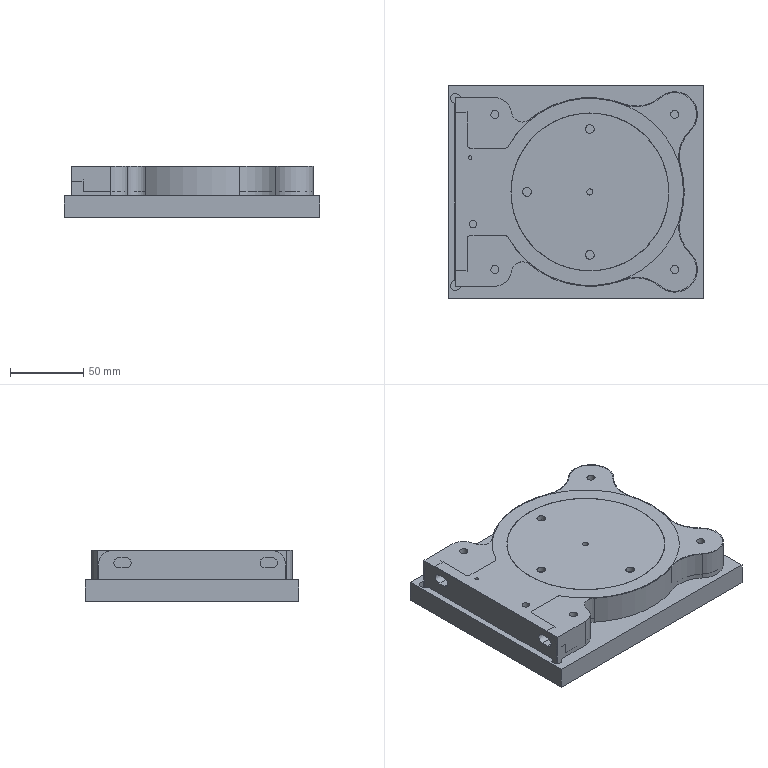NC program | NX | posted with a generic post | part box 175 x 146 x 35 mm
Lines 4709 to 5827 of 35144:
(深度开粗_COPY , TOOL : D6)
N9278 T04 M6
N9280 G54
N9282 G17 G0 G90 X-65.994 Y19.5 S9000 M3
N9284 G43 Z20. H4
N9286 Z0.
N9288 G94 G1 Z-0.5 F2500.
N9290 G3 X-68.994 Y22.5 R3.
N9292 G1 X-71.
N9294 Y20.494
N9296 G3 X-68. Y17.494 R3.
N9298 G1 Z0.
N9300 G0 X-65.994 Y19.5 Z-0.5
N9302 G1 Z-1.
N9304 G3 X-68.994 Y22.5 R3.
N9306 G1 X-71.
N9308 Y20.494
N9310 G3 X-68. Y17.494 R3.
N9312 G1 Z-0.5
N9314 G0 X-65.994 Y19.5 Z-1.
N9316 G1 Z-1.5
N9318 G3 X-68.994 Y22.5 R3.
N9320 G1 X-71.
N9322 Y20.494
N9324 G3 X-68. Y17.494 R3.
N9326 G1 Z-1.
N9328 G0 X-65.994 Y19.5 Z-1.5
N9330 G1 Z-2.
N9332 G3 X-68.994 Y22.5 R3.
N9334 G1 X-71.
N9336 Y20.494
N9338 G3 X-68. Y17.494 R3.
N9340 G1 Z-1.5
N9342 G0 X-65.994 Y19.5 Z-2.
N9344 G1 Z-2.5
N9346 G3 X-68.994 Y22.5 R3.
N9348 G1 X-71.
N9350 Y20.494
N9352 G3 X-68. Y17.494 R3.
N9354 G1 Z-2.
N9356 G0 X-65.994 Y19.5 Z-2.5
N9358 G1 Z-3.
N9360 G3 X-68.994 Y22.5 R3.
N9362 G1 X-71.
N9364 Y20.494
N9366 G3 X-68. Y17.494 R3.
N9368 G1 Z-2.5
N9370 G0 X-65.994 Y19.5 Z-3.
N9372 G1 Z-3.5
N9374 G3 X-68.994 Y22.5 R3.
N9376 G1 X-71.
N9378 Y20.494
N9380 G3 X-68. Y17.494 R3.
N9382 G1 Z-3.
N9384 G0 X-65.994 Y19.5 Z-3.5
N9386 G1 Z-4.
N9388 G3 X-68.994 Y22.5 R3.
N9390 G1 X-71.
N9392 Y20.494
N9394 G3 X-68. Y17.494 R3.
N9396 G1 Z-3.5
N9398 G0 X-65.994 Y19.5 Z-4.
N9400 G1 Z-4.5
N9402 G3 X-68.994 Y22.5 R3.
N9404 G1 X-71.
N9406 Y20.494
N9408 G3 X-68. Y17.494 R3.
N9410 G1 Z-4.
N9412 G0 X-65.994 Y19.5 Z-4.5
N9414 G1 Z-5.
N9416 G3 X-68.994 Y22.5 R3.
N9418 G1 X-71.
N9420 Y20.494
N9422 G3 X-68. Y17.494 R3.
N9424 G1 Z-4.5
N9426 G0 X-65.994 Y19.5 Z-5.
N9428 G1 Z-5.5
N9430 G3 X-68.994 Y22.5 R3.
N9432 G1 X-71.
N9434 Y20.494
N9436 G3 X-68. Y17.494 R3.
N9438 G1 Z-5.
N9440 G0 X-65.994 Y19.5 Z-5.5
N9442 G1 Z-6.
N9444 G3 X-68.994 Y22.5 R3.
N9446 G1 X-71.
N9448 Y20.494
N9450 G3 X-68. Y17.494 R3.
N9452 G1 Z-5.5
N9454 G0 X-65.994 Y19.5 Z-6.
N9456 G1 Z-6.5
N9458 G3 X-68.994 Y22.5 R3.
N9460 G1 X-71.
N9462 Y20.494
N9464 G3 X-68. Y17.494 R3.
N9466 G1 Z-6.
N9468 G0 X-65.994 Y19.5 Z-6.5
N9470 G1 Z-7.
N9472 G3 X-68.994 Y22.5 R3.
N9474 G1 X-71.
N9476 Y20.494
N9478 G3 X-68. Y17.494 R3.
N9480 G1 Z-6.5
N9482 G0 X-65.994 Y19.5 Z-7.
N9484 G1 Z-7.5
N9486 G3 X-68.994 Y22.5 R3.
N9488 G1 X-71.
N9490 Y20.494
N9492 G3 X-68. Y17.494 R3.
N9494 G1 Z-7.
N9496 G0 X-65.994 Y19.5 Z-7.5
N9498 G1 Z-8.
N9500 G3 X-68.994 Y22.5 R3.
N9502 G1 X-71.
N9504 Y20.494
N9506 G3 X-68. Y17.494 R3.
N9508 G1 Z-7.5
N9510 G0 X-65.994 Y19.5 Z-8.
N9512 G1 Z-8.5
N9514 G3 X-68.994 Y22.5 R3.
N9516 G1 X-71.
N9518 Y20.494
N9520 G3 X-68. Y17.494 R3.
N9522 G1 Z-8.
N9524 G0 X-65.994 Y19.5 Z-8.5
N9526 G1 Z-9.
N9528 G3 X-68.994 Y22.5 R3.
N9530 G1 X-71.
N9532 Y20.494
N9534 G3 X-68. Y17.494 R3.
N9536 G1 Z-8.5
N9538 G0 X-65.994 Y19.5 Z-9.
N9540 G1 Z-9.5
N9542 G3 X-68.994 Y22.5 R3.
N9544 G1 X-71.
N9546 Y20.494
N9548 G3 X-68. Y17.494 R3.
N9550 G1 Z-9.
N9552 G0 X-65.994 Y19.5 Z-9.5
N9554 G1 Z-10.
N9556 G3 X-68.994 Y22.5 R3.
N9558 G1 X-71.
N9560 Y20.494
N9562 G3 X-68. Y17.494 R3.
N9564 G1 Z-9.5
N9566 G0 X-65.994 Y19.5 Z-10.
N9568 G1 Z-10.5
N9570 G3 X-68.994 Y22.5 R3.
N9572 G1 X-71.
N9574 Y20.494
N9576 G3 X-68. Y17.494 R3.
N9578 G1 Z-10.
N9580 G0 X-65.994 Y19.5 Z-10.5
N9582 G1 Z-11.
N9584 G3 X-68.994 Y22.5 R3.
N9586 G1 X-71.
N9588 Y20.494
N9590 G3 X-68. Y17.494 R3.
N9592 G1 Z-10.5
N9594 G0 X-65.994 Y19.5 Z-11.
N9596 G1 Z-11.5
N9598 G3 X-68.994 Y22.5 R3.
N9600 G1 X-71.
N9602 Y20.494
N9604 G3 X-68. Y17.494 R3.
N9606 G1 Z-11.
N9608 G0 X-65.994 Y19.5 Z-11.5
N9610 G1 Z-12.
N9612 G3 X-68.994 Y22.5 R3.
N9614 G1 X-71.
N9616 Y20.494
N9618 G3 X-68. Y17.494 R3.
N9620 G1 Z-11.5
N9622 G0 X-65.994 Y19.5 Z-12.
N9624 G1 Z-12.5
N9626 G3 X-68.994 Y22.5 R3.
N9628 G1 X-71.
N9630 Y20.494
N9632 G3 X-68. Y17.494 R3.
N9634 G1 Z-12.
N9636 G0 X-65.994 Y19.5 Z-12.5
N9638 G1 Z-13.
N9640 G3 X-68.994 Y22.5 R3.
N9642 G1 X-71.
N9644 Y20.494
N9646 G3 X-68. Y17.494 R3.
N9648 G1 Z-12.5
N9650 G0 X-65.994 Y19.5 Z-13.
N9652 G1 Z-13.5
N9654 G3 X-68.994 Y22.5 R3.
N9656 G1 X-71.
N9658 Y20.494
N9660 G3 X-68. Y17.494 R3.
N9662 G1 Z-13.
N9664 G0 X-65.994 Y19.5 Z-13.5
N9666 G1 Z-14.
N9668 G3 X-68.994 Y22.5 R3.
N9670 G1 X-71.
N9672 Y20.494
N9674 G3 X-68. Y17.494 R3.
N9676 G1 Z-13.5
N9678 G0 X-65.994 Y19.5 Z-14.
N9680 G1 Z-14.5
N9682 G3 X-68.994 Y22.5 R3.
N9684 G1 X-71.
N9686 Y20.494
N9688 G3 X-68. Y17.494 R3.
N9690 G1 Z-14.
N9692 G0 X-65.994 Y19.5 Z-14.5
N9694 G1 Z-15.
N9696 G3 X-68.994 Y22.5 R3.
N9698 G1 X-71.
N9700 Y20.494
N9702 G3 X-68. Y17.494 R3.
N9704 G1 Z-14.5
N9706 G0 X-65.994 Y19.5 Z-15.
N9708 G1 Z-15.5
N9710 G3 X-68.994 Y22.5 R3.
N9712 G1 X-71.
N9714 Y20.494
N9716 G3 X-68. Y17.494 R3.
N9718 G1 Z-15.
N9720 G0 X-65.994 Y19.5 Z-15.5
N9722 G1 Z-16.
N9724 G3 X-68.994 Y22.5 R3.
N9726 G1 X-71.
N9728 Y20.494
N9730 G3 X-68. Y17.494 R3.
N9732 G1 Z-15.5
N9734 G0 X-65.994 Y19.5 Z-16.
N9736 G1 Z-16.5
N9738 G3 X-68.994 Y22.5 R3.
N9740 G1 X-71.
N9742 Y20.494
N9744 G3 X-68. Y17.494 R3.
N9746 G1 Z-16.
N9748 G0 X-65.994 Y19.5 Z-16.5
N9750 G1 Z-17.
N9752 G3 X-68.994 Y22.5 R3.
N9754 G1 X-71.
N9756 Y20.494
N9758 G3 X-68. Y17.494 R3.
N9760 G1 Z-16.5
N9762 G0 X-65.994 Y19.5 Z-17.
N9764 G1 Z-17.5
N9766 G3 X-68.994 Y22.5 R3.
N9768 G1 X-71.
N9770 Y20.494
N9772 G3 X-68. Y17.494 R3.
N9774 G1 Z-17.
N9776 G0 X-65.994 Y19.5 Z-17.5
N9778 G1 Z-18.
N9780 G3 X-68.994 Y22.5 R3.
N9782 G1 X-71.
N9784 Y20.494
N9786 G3 X-68. Y17.494 R3.
N9788 G1 Z-17.5
N9790 G0 X-65.994 Y19.5 Z-18.
N9792 G1 Z-18.5
N9794 G3 X-68.994 Y22.5 R3.
N9796 G1 X-71.
N9798 Y20.494
N9800 G3 X-68. Y17.494 R3.
N9802 G1 Z-18.
N9804 G0 X-65.994 Y19.5 Z-18.5
N9806 G1 Z-19.
N9808 G3 X-68.994 Y22.5 R3.
N9810 G1 X-71.
N9812 Y20.494
N9814 G3 X-68. Y17.494 R3.
N9816 G1 Z-18.5
N9818 G0 X-65.994 Y19.5 Z-18.8
N9820 G1 Z-19.3
N9822 G3 X-68.994 Y22.5 R3.
N9824 G1 X-71.
N9826 Y20.494
N9828 G3 X-68. Y17.494 R3.
N9830 G1 Z-18.8
N9832 G0 X-65.994 Y11.523 Z-19.15
N9834 G1 Z-19.65
N9836 G3 X-68.994 Y14.523 R3.
N9838 G1 X-71.
N9840 Y12.517
N9842 G3 X-68. Y9.517 R3.
N9844 G1 Z-19.15
N9846 G0 X-65.994 Y11.5 Z-19.5
N9848 G1 Z-20.
N9850 G3 X-68.994 Y14.5 R3.
N9852 G1 X-71.
N9854 Y12.494
N9856 G3 X-68. Y9.494 R3.
N9858 G1 Z-19.5
N9860 G0 Z20.
N9862 X-62. Y17.494
N9864 Z-1.
N9866 G1 Z-1.5
N9868 G3 X-59. Y20.494 R3.
N9870 G1 Y22.5
N9872 X-61.006
N9874 G3 X-64.006 Y19.5 R3.
N9876 G1 Z-1.
N9878 G0 X-62. Y17.494 Z-1.5
N9880 G1 Z-2.
N9882 G3 X-59. Y20.494 R3.
N9884 G1 Y22.5
N9886 X-61.006
N9888 G3 X-64.006 Y19.5 R3.
N9890 G1 Z-1.5
N9892 G0 X-62. Y17.494 Z-2.
N9894 G1 Z-2.5
N9896 G3 X-59. Y20.494 R3.
N9898 G1 Y22.5
N9900 X-61.006
N9902 G3 X-64.006 Y19.5 R3.
N9904 G1 Z-2.
N9906 G0 X-62. Y17.494 Z-2.5
N9908 G1 Z-3.
N9910 G3 X-59. Y20.494 R3.
N9912 G1 Y22.5
N9914 X-61.006
N9916 G3 X-64.006 Y19.5 R3.
N9918 G1 Z-2.5
N9920 G0 X-62. Y17.494 Z-3.
N9922 G1 Z-3.5
N9924 G3 X-59. Y20.494 R3.
N9926 G1 Y22.5
N9928 X-61.006
N9930 G3 X-64.006 Y19.5 R3.
N9932 G1 Z-3.
N9934 G0 X-62. Y17.494 Z-3.5
N9936 G1 Z-4.
N9938 G3 X-59. Y20.494 R3.
N9940 G1 Y22.5
N9942 X-61.006
N9944 G3 X-64.006 Y19.5 R3.
N9946 G1 Z-3.5
N9948 G0 X-62. Y17.494 Z-4.
N9950 G1 Z-4.5
N9952 G3 X-59. Y20.494 R3.
N9954 G1 Y22.5
N9956 X-61.006
N9958 G3 X-64.006 Y19.5 R3.
N9960 G1 Z-4.
N9962 G0 X-62. Y17.494 Z-4.5
N9964 G1 Z-5.
N9966 G3 X-59. Y20.494 R3.
N9968 G1 Y22.5
N9970 X-61.006
N9972 G3 X-64.006 Y19.5 R3.
N9974 G1 Z-4.5
N9976 G0 X-62. Y17.494 Z-5.
N9978 G1 Z-5.5
N9980 G3 X-59. Y20.494 R3.
N9982 G1 Y22.5
N9984 X-61.006
N9986 G3 X-64.006 Y19.5 R3.
N9988 G1 Z-5.
N9990 G0 X-62. Y17.494 Z-5.5
N9992 G1 Z-6.
N9994 G3 X-59. Y20.494 R3.
N9996 G1 Y22.5
N9998 X-61.006
N10000 G3 X-64.006 Y19.5 R3.
N10002 G1 Z-5.5
N10004 G0 X-62. Y17.494 Z-6.
N10006 G1 Z-6.5
N10008 G3 X-59. Y20.494 R3.
N10010 G1 Y22.5
N10012 X-61.006
N10014 G3 X-64.006 Y19.5 R3.
N10016 G1 Z-6.
N10018 G0 X-62. Y17.494 Z-6.5
N10020 G1 Z-7.
N10022 G3 X-59. Y20.494 R3.
N10024 G1 Y22.5
N10026 X-61.006
N10028 G3 X-64.006 Y19.5 R3.
N10030 G1 Z-6.5
N10032 G0 X-62. Y17.494 Z-7.
N10034 G1 Z-7.5
N10036 G3 X-59. Y20.494 R3.
N10038 G1 Y22.5
N10040 X-61.006
N10042 G3 X-64.006 Y19.5 R3.
N10044 G1 Z-7.
N10046 G0 X-62. Y17.494 Z-7.5
N10048 G1 Z-8.
N10050 G3 X-59. Y20.494 R3.
N10052 G1 Y22.5
N10054 X-61.006
N10056 G3 X-64.006 Y19.5 R3.
N10058 G1 Z-7.5
N10060 G0 X-62. Y17.494 Z-8.
N10062 G1 Z-8.5
N10064 G3 X-59. Y20.494 R3.
N10066 G1 Y22.5
N10068 X-61.006
N10070 G3 X-64.006 Y19.5 R3.
N10072 G1 Z-8.
N10074 G0 X-62. Y17.494 Z-8.5
N10076 G1 Z-9.
N10078 G3 X-59. Y20.494 R3.
N10080 G1 Y22.5
N10082 X-61.006
N10084 G3 X-64.006 Y19.5 R3.
N10086 G1 Z-8.5
N10088 G0 X-62. Y17.494 Z-9.
N10090 G1 Z-9.5
N10092 G3 X-59. Y20.494 R3.
N10094 G1 Y22.5
N10096 X-61.006
N10098 G3 X-64.006 Y19.5 R3.
N10100 G1 Z-9.
N10102 G0 X-62. Y17.494 Z-9.5
N10104 G1 Z-10.
N10106 G3 X-59. Y20.494 R3.
N10108 G1 Y22.5
N10110 X-61.006
N10112 G3 X-64.006 Y19.5 R3.
N10114 G1 Z-9.5
N10116 G0 X-62. Y17.494 Z-10.
N10118 G1 Z-10.5
N10120 G3 X-59. Y20.494 R3.
N10122 G1 Y22.5
N10124 X-61.006
N10126 G3 X-64.006 Y19.5 R3.
N10128 G1 Z-10.
N10130 G0 X-62. Y17.494 Z-10.5
N10132 G1 Z-11.
N10134 G3 X-59. Y20.494 R3.
N10136 G1 Y22.5
N10138 X-61.006
N10140 G3 X-64.006 Y19.5 R3.
N10142 G1 Z-10.5
N10144 G0 X-62. Y17.494 Z-11.
N10146 G1 Z-11.5
N10148 G3 X-59. Y20.494 R3.
N10150 G1 Y22.5
N10152 X-61.006
N10154 G3 X-64.006 Y19.5 R3.
N10156 G1 Z-11.
N10158 G0 X-62. Y17.494 Z-11.5
N10160 G1 Z-12.
N10162 G3 X-59. Y20.494 R3.
N10164 G1 Y22.5
N10166 X-61.006
N10168 G3 X-64.006 Y19.5 R3.
N10170 G1 Z-11.5
N10172 G0 X-62. Y17.494 Z-12.
N10174 G1 Z-12.5
N10176 G3 X-59. Y20.494 R3.
N10178 G1 Y22.5
N10180 X-61.006
N10182 G3 X-64.006 Y19.5 R3.
N10184 G1 Z-12.
N10186 G0 X-62. Y17.494 Z-12.5
N10188 G1 Z-13.
N10190 G3 X-59. Y20.494 R3.
N10192 G1 Y22.5
N10194 X-61.006
N10196 G3 X-64.006 Y19.5 R3.
N10198 G1 Z-12.5
N10200 G0 X-62. Y17.494 Z-13.
N10202 G1 Z-13.5
N10204 G3 X-59. Y20.494 R3.
N10206 G1 Y22.5
N10208 X-61.006
N10210 G3 X-64.006 Y19.5 R3.
N10212 G1 Z-13.
N10214 G0 X-62. Y17.494 Z-13.5
N10216 G1 Z-14.
N10218 G3 X-59. Y20.494 R3.
N10220 G1 Y22.5
N10222 X-61.006
N10224 G3 X-64.006 Y19.5 R3.
N10226 G1 Z-13.5
N10228 G0 X-62. Y17.494 Z-14.
N10230 G1 Z-14.5
N10232 G3 X-59. Y20.494 R3.
N10234 G1 Y22.5
N10236 X-61.006
N10238 G3 X-64.006 Y19.5 R3.
N10240 G1 Z-14.
N10242 G0 X-62. Y17.494 Z-14.5
N10244 G1 Z-15.
N10246 G3 X-59. Y20.494 R3.
N10248 G1 Y22.5
N10250 X-61.006
N10252 G3 X-64.006 Y19.5 R3.
N10254 G1 Z-14.5
N10256 G0 X-62. Y17.494 Z-15.
N10258 G1 Z-15.5
N10260 G3 X-59. Y20.494 R3.
N10262 G1 Y22.5
N10264 X-61.006
N10266 G3 X-64.006 Y19.5 R3.
N10268 G1 Z-15.
N10270 G0 X-62. Y17.494 Z-15.5
N10272 G1 Z-16.
N10274 G3 X-59. Y20.494 R3.
N10276 G1 Y22.5
N10278 X-61.006
N10280 G3 X-64.006 Y19.5 R3.
N10282 G1 Z-15.5
N10284 G0 X-62. Y17.494 Z-16.
N10286 G1 Z-16.5
N10288 G3 X-59. Y20.494 R3.
N10290 G1 Y22.5
N10292 X-61.006
N10294 G3 X-64.006 Y19.5 R3.
N10296 G1 Z-16.
N10298 G0 X-62. Y17.494 Z-16.5
N10300 G1 Z-17.
N10302 G3 X-59. Y20.494 R3.
N10304 G1 Y22.5
N10306 X-61.006
N10308 G3 X-64.006 Y19.5 R3.
N10310 G1 Z-16.5
N10312 G0 X-62. Y17.494 Z-17.
N10314 G1 Z-17.5
N10316 G3 X-59. Y20.494 R3.
N10318 G1 Y22.5
N10320 X-61.006
N10322 G3 X-64.006 Y19.5 R3.
N10324 G1 Z-17.
N10326 G0 X-62. Y17.494 Z-17.5
N10328 G1 Z-18.
N10330 G3 X-59. Y20.494 R3.
N10332 G1 Y22.5
N10334 X-61.006
N10336 G3 X-64.006 Y19.5 R3.
N10338 G1 Z-17.5
N10340 G0 X-62. Y17.494 Z-18.
N10342 G1 Z-18.5
N10344 G3 X-59. Y20.494 R3.
N10346 G1 Y22.5
N10348 X-61.006
N10350 G3 X-64.006 Y19.5 R3.
N10352 G1 Z-18.
N10354 G0 X-62. Y17.494 Z-18.5
N10356 G1 Z-19.
N10358 G3 X-59. Y20.494 R3.
N10360 G1 Y22.5
N10362 X-61.006
N10364 G3 X-64.006 Y19.5 R3.
N10366 G1 Z-18.5
N10368 G0 X-62. Y17.494 Z-18.8
N10370 G1 Z-19.3
N10372 G3 X-59. Y20.494 R3.
N10374 G1 Y22.5
N10376 X-61.006
N10378 G3 X-64.006 Y19.5 R3.
N10380 G1 Z-18.8
N10382 G0 X-62. Y17.141 Z-19.15
N10384 G1 Z-19.65
N10386 G3 X-59. Y20.141 R3.
N10388 G1 Y22.5
N10390 X-63.023
N10392 Y20.141
N10394 G3 X-60.023 Y17.141 R3.
N10396 G1 Z-19.15
N10398 G0 X-62. Y14.906 Z-19.5
N10400 G1 Z-20.
N10402 G3 X-59. Y17.906 R3.
N10404 G1 Y22.5
N10406 X-63.
N10408 Y18.335
N10410 G3 X-60. Y15.335 R3.
N10412 G1 Z-19.5
N10414 G0 Z20.
N10416 X-68. Y-17.494
N10418 Z0.
N10420 G1 Z-0.5
N10422 G3 X-71. Y-20.494 R3.
N10424 G1 Y-22.5
N10426 X-68.994
N10428 G3 X-65.994 Y-19.5 R3.
N10430 G1 Z0.
N10432 G0 X-68. Y-17.494 Z-0.5
N10434 G1 Z-1.
N10436 G3 X-71. Y-20.494 R3.
N10438 G1 Y-22.5
N10440 X-68.994
N10442 G3 X-65.994 Y-19.5 R3.
N10444 G1 Z-0.5
N10446 G0 X-68. Y-17.494 Z-1.
N10448 G1 Z-1.5
N10450 G3 X-71. Y-20.494 R3.
N10452 G1 Y-22.5
N10454 X-68.994
N10456 G3 X-65.994 Y-19.5 R3.
N10458 G1 Z-1.
N10460 G0 X-68. Y-17.494 Z-1.5
N10462 G1 Z-2.
N10464 G3 X-71. Y-20.494 R3.
N10466 G1 Y-22.5
N10468 X-68.994
N10470 G3 X-65.994 Y-19.5 R3.
N10472 G1 Z-1.5
N10474 G0 X-68. Y-17.494 Z-2.
N10476 G1 Z-2.5
N10478 G3 X-71. Y-20.494 R3.
N10480 G1 Y-22.5
N10482 X-68.994
N10484 G3 X-65.994 Y-19.5 R3.
N10486 G1 Z-2.
N10488 G0 X-68. Y-17.494 Z-2.5
N10490 G1 Z-3.
N10492 G3 X-71. Y-20.494 R3.
N10494 G1 Y-22.5
N10496 X-68.994
N10498 G3 X-65.994 Y-19.5 R3.
N10500 G1 Z-2.5
N10502 G0 X-68. Y-17.494 Z-3.
N10504 G1 Z-3.5
N10506 G3 X-71. Y-20.494 R3.
N10508 G1 Y-22.5
N10510 X-68.994
N10512 G3 X-65.994 Y-19.5 R3.
N10514 G1 Z-3.
N10516 G0 X-68. Y-17.494 Z-3.5
N10518 G1 Z-4.
N10520 G3 X-71. Y-20.494 R3.
N10522 G1 Y-22.5
N10524 X-68.994
N10526 G3 X-65.994 Y-19.5 R3.
N10528 G1 Z-3.5
N10530 G0 X-68. Y-17.494 Z-4.
N10532 G1 Z-4.5
N10534 G3 X-71. Y-20.494 R3.
N10536 G1 Y-22.5
N10538 X-68.994
N10540 G3 X-65.994 Y-19.5 R3.
N10542 G1 Z-4.
N10544 G0 X-68. Y-17.494 Z-4.5
N10546 G1 Z-5.
N10548 G3 X-71. Y-20.494 R3.
N10550 G1 Y-22.5
N10552 X-68.994
N10554 G3 X-65.994 Y-19.5 R3.
N10556 G1 Z-4.5
N10558 G0 X-68. Y-17.494 Z-5.
N10560 G1 Z-5.5
N10562 G3 X-71. Y-20.494 R3.
N10564 G1 Y-22.5
N10566 X-68.994
N10568 G3 X-65.994 Y-19.5 R3.
N10570 G1 Z-5.
N10572 G0 X-68. Y-17.494 Z-5.5
N10574 G1 Z-6.
N10576 G3 X-71. Y-20.494 R3.
N10578 G1 Y-22.5
N10580 X-68.994
N10582 G3 X-65.994 Y-19.5 R3.
N10584 G1 Z-5.5
N10586 G0 X-68. Y-17.494 Z-6.
N10588 G1 Z-6.5
N10590 G3 X-71. Y-20.494 R3.
N10592 G1 Y-22.5
N10594 X-68.994
N10596 G3 X-65.994 Y-19.5 R3.
N10598 G1 Z-6.
N10600 G0 X-68. Y-17.494 Z-6.5
N10602 G1 Z-7.
N10604 G3 X-71. Y-20.494 R3.
N10606 G1 Y-22.5
N10608 X-68.994
N10610 G3 X-65.994 Y-19.5 R3.
N10612 G1 Z-6.5
N10614 G0 X-68. Y-17.494 Z-7.
N10616 G1 Z-7.5
N10618 G3 X-71. Y-20.494 R3.
N10620 G1 Y-22.5
N10622 X-68.994
N10624 G3 X-65.994 Y-19.5 R3.
N10626 G1 Z-7.
N10628 G0 X-68. Y-17.494 Z-7.5
N10630 G1 Z-8.
N10632 G3 X-71. Y-20.494 R3.
N10634 G1 Y-22.5
N10636 X-68.994
N10638 G3 X-65.994 Y-19.5 R3.
N10640 G1 Z-7.5
N10642 G0 X-68. Y-17.494 Z-8.
N10644 G1 Z-8.5
N10646 G3 X-71. Y-20.494 R3.
N10648 G1 Y-22.5
N10650 X-68.994
N10652 G3 X-65.994 Y-19.5 R3.
N10654 G1 Z-8.
N10656 G0 X-68. Y-17.494 Z-8.5
N10658 G1 Z-9.
N10660 G3 X-71. Y-20.494 R3.
N10662 G1 Y-22.5
N10664 X-68.994
N10666 G3 X-65.994 Y-19.5 R3.
N10668 G1 Z-8.5
N10670 G0 X-68. Y-17.494 Z-9.
N10672 G1 Z-9.5
N10674 G3 X-71. Y-20.494 R3.
N10676 G1 Y-22.5
N10678 X-68.994
N10680 G3 X-65.994 Y-19.5 R3.
N10682 G1 Z-9.
N10684 G0 X-68. Y-17.494 Z-9.5
N10686 G1 Z-10.
N10688 G3 X-71. Y-20.494 R3.
N10690 G1 Y-22.5
N10692 X-68.994
N10694 G3 X-65.994 Y-19.5 R3.
N10696 G1 Z-9.5
N10698 G0 X-68. Y-17.494 Z-10.
N10700 G1 Z-10.5
N10702 G3 X-71. Y-20.494 R3.
N10704 G1 Y-22.5
N10706 X-68.994
N10708 G3 X-65.994 Y-19.5 R3.
N10710 G1 Z-10.
N10712 G0 X-68. Y-17.494 Z-10.5
N10714 G1 Z-11.
N10716 G3 X-71. Y-20.494 R3.
N10718 G1 Y-22.5
N10720 X-68.994
N10722 G3 X-65.994 Y-19.5 R3.
N10724 G1 Z-10.5
N10726 G0 X-68. Y-17.494 Z-11.
N10728 G1 Z-11.5
N10730 G3 X-71. Y-20.494 R3.
N10732 G1 Y-22.5
N10734 X-68.994
N10736 G3 X-65.994 Y-19.5 R3.
N10738 G1 Z-11.
N10740 G0 X-68. Y-17.494 Z-11.5
N10742 G1 Z-12.
N10744 G3 X-71. Y-20.494 R3.
N10746 G1 Y-22.5
N10748 X-68.994
N10750 G3 X-65.994 Y-19.5 R3.
N10752 G1 Z-11.5
N10754 G0 X-68. Y-17.494 Z-12.
N10756 G1 Z-12.5
N10758 G3 X-71. Y-20.494 R3.
N10760 G1 Y-22.5
N10762 X-68.994
N10764 G3 X-65.994 Y-19.5 R3.
N10766 G1 Z-12.
N10768 G0 X-68. Y-17.494 Z-12.5
N10770 G1 Z-13.
N10772 G3 X-71. Y-20.494 R3.
N10774 G1 Y-22.5
N10776 X-68.994
N10778 G3 X-65.994 Y-19.5 R3.
N10780 G1 Z-12.5
N10782 G0 X-68. Y-17.494 Z-13.
N10784 G1 Z-13.5
N10786 G3 X-71. Y-20.494 R3.
N10788 G1 Y-22.5
N10790 X-68.994
N10792 G3 X-65.994 Y-19.5 R3.
N10794 G1 Z-13.
N10796 G0 X-68. Y-17.494 Z-13.5
N10798 G1 Z-14.
N10800 G3 X-71. Y-20.494 R3.
N10802 G1 Y-22.5
N10804 X-68.994
N10806 G3 X-65.994 Y-19.5 R3.
N10808 G1 Z-13.5
N10810 G0 X-68. Y-17.494 Z-14.
N10812 G1 Z-14.5
N10814 G3 X-71. Y-20.494 R3.
N10816 G1 Y-22.5
N10818 X-68.994
N10820 G3 X-65.994 Y-19.5 R3.
N10822 G1 Z-14.
N10824 G0 X-68. Y-17.494 Z-14.5
N10826 G1 Z-15.
N10828 G3 X-71. Y-20.494 R3.
N10830 G1 Y-22.5
N10832 X-68.994
N10834 G3 X-65.994 Y-19.5 R3.
N10836 G1 Z-14.5
N10838 G0 X-68. Y-17.494 Z-15.
N10840 G1 Z-15.5
N10842 G3 X-71. Y-20.494 R3.
N10844 G1 Y-22.5
N10846 X-68.994
N10848 G3 X-65.994 Y-19.5 R3.
N10850 G1 Z-15.
N10852 G0 X-68. Y-17.494 Z-15.5
N10854 G1 Z-16.
N10856 G3 X-71. Y-20.494 R3.
N10858 G1 Y-22.5
N10860 X-68.994
N10862 G3 X-65.994 Y-19.5 R3.
N10864 G1 Z-15.5
N10866 G0 X-68. Y-17.494 Z-16.
N10868 G1 Z-16.5
N10870 G3 X-71. Y-20.494 R3.
N10872 G1 Y-22.5
N10874 X-68.994
N10876 G3 X-65.994 Y-19.5 R3.
N10878 G1 Z-16.
N10880 G0 X-68. Y-17.494 Z-16.5
N10882 G1 Z-17.
N10884 G3 X-71. Y-20.494 R3.
N10886 G1 Y-22.5
N10888 X-68.994
N10890 G3 X-65.994 Y-19.5 R3.
N10892 G1 Z-16.5
N10894 G0 X-68. Y-17.494 Z-17.
N10896 G1 Z-17.5
N10898 G3 X-71. Y-20.494 R3.
N10900 G1 Y-22.5
N10902 X-68.994
N10904 G3 X-65.994 Y-19.5 R3.
N10906 G1 Z-17.
N10908 G0 X-68. Y-17.494 Z-17.5
N10910 G1 Z-18.
N10912 G3 X-71. Y-20.494 R3.
N10914 G1 Y-22.5
N10916 X-68.994
N10918 G3 X-65.994 Y-19.5 R3.
N10920 G1 Z-17.5
N10922 G0 X-68. Y-17.494 Z-18.
N10924 G1 Z-18.5
N10926 G3 X-71. Y-20.494 R3.
N10928 G1 Y-22.5
N10930 X-68.994
N10932 G3 X-65.994 Y-19.5 R3.
N10934 G1 Z-18.
N10936 G0 X-68. Y-17.494 Z-18.5
N10938 G1 Z-19.
N10940 G3 X-71. Y-20.494 R3.
N10942 G1 Y-22.5
N10944 X-68.994
N10946 G3 X-65.994 Y-19.5 R3.
N10948 G1 Z-18.5
N10950 G0 X-68. Y-17.494 Z-18.8
N10952 G1 Z-19.3
N10954 G3 X-71. Y-20.494 R3.
N10956 G1 Y-22.5
N10958 X-68.994
N10960 G3 X-65.994 Y-19.5 R3.
N10962 G1 Z-18.8
N10964 G0 X-68. Y-17.494 Z-19.15
N10966 G1 Z-19.65
N10968 G3 X-71. Y-20.494 R3.
N10970 G1 Y-22.5
N10972 X-68.994
N10974 G3 X-65.994 Y-19.5 R3.
N10976 G1 Z-19.15
N10978 G0 X-68. Y-17.494 Z-19.5
N10980 G1 Z-20.
N10982 G3 X-71. Y-20.494 R3.
N10984 G1 Y-22.5
N10986 X-68.994
N10988 G3 X-65.994 Y-19.5 R3.
N10990 G1 Z-19.5
N10992 G0 Z20.
N10994 X-64.006
N10996 Z-1.
N10998 G1 Z-1.5
N11000 G3 X-61.006 Y-22.5 R3.
N11002 G1 X-59.
N11004 Y-20.494
N11006 G3 X-62. Y-17.494 R3.
N11008 G1 Z-1.
N11010 G0 X-64.006 Y-19.5 Z-1.5
N11012 G1 Z-2.
N11014 G3 X-61.006 Y-22.5 R3.
N11016 G1 X-59.
N11018 Y-20.494
N11020 G3 X-62. Y-17.494 R3.
N11022 G1 Z-1.5
N11024 G0 X-64.006 Y-19.5 Z-2.
N11026 G1 Z-2.5
N11028 G3 X-61.006 Y-22.5 R3.
N11030 G1 X-59.
N11032 Y-20.494
N11034 G3 X-62. Y-17.494 R3.
N11036 G1 Z-2.
N11038 G0 X-64.006 Y-19.5 Z-2.5
N11040 G1 Z-3.
N11042 G3 X-61.006 Y-22.5 R3.
N11044 G1 X-59.
N11046 Y-20.494
N11048 G3 X-62. Y-17.494 R3.
N11050 G1 Z-2.5
N11052 G0 X-64.006 Y-19.5 Z-3.
N11054 G1 Z-3.5
N11056 G3 X-61.006 Y-22.5 R3.
N11058 G1 X-59.
N11060 Y-20.494
N11062 G3 X-62. Y-17.494 R3.
N11064 G1 Z-3.
N11066 G0 X-64.006 Y-19.5 Z-3.5
N11068 G1 Z-4.
N11070 G3 X-61.006 Y-22.5 R3.
N11072 G1 X-59.
N11074 Y-20.494
N11076 G3 X-62. Y-17.494 R3.
N11078 G1 Z-3.5
N11080 G0 X-64.006 Y-19.5 Z-4.
N11082 G1 Z-4.5
N11084 G3 X-61.006 Y-22.5 R3.
N11086 G1 X-59.
N11088 Y-20.494
N11090 G3 X-62. Y-17.494 R3.
N11092 G1 Z-4.
N11094 G0 X-64.006 Y-19.5 Z-4.5
N11096 G1 Z-5.
N11098 G3 X-61.006 Y-22.5 R3.
N11100 G1 X-59.
N11102 Y-20.494
N11104 G3 X-62. Y-17.494 R3.
N11106 G1 Z-4.5
N11108 G0 X-64.006 Y-19.5 Z-5.
N11110 G1 Z-5.5
N11112 G3 X-61.006 Y-22.5 R3.
N11114 G1 X-59.
N11116 Y-20.494
N11118 G3 X-62. Y-17.494 R3.
N11120 G1 Z-5.
N11122 G0 X-64.006 Y-19.5 Z-5.5
N11124 G1 Z-6.
N11126 G3 X-61.006 Y-22.5 R3.
N11128 G1 X-59.
N11130 Y-20.494
N11132 G3 X-62. Y-17.494 R3.
N11134 G1 Z-5.5
N11136 G0 X-64.006 Y-19.5 Z-6.
N11138 G1 Z-6.5
N11140 G3 X-61.006 Y-22.5 R3.
N11142 G1 X-59.
N11144 Y-20.494
N11146 G3 X-62. Y-17.494 R3.
N11148 G1 Z-6.
N11150 G0 X-64.006 Y-19.5 Z-6.5
N11152 G1 Z-7.
N11154 G3 X-61.006 Y-22.5 R3.
N11156 G1 X-59.
N11158 Y-20.494
N11160 G3 X-62. Y-17.494 R3.
N11162 G1 Z-6.5
N11164 G0 X-64.006 Y-19.5 Z-7.
N11166 G1 Z-7.5
N11168 G3 X-61.006 Y-22.5 R3.
N11170 G1 X-59.
N11172 Y-20.494
N11174 G3 X-62. Y-17.494 R3.
N11176 G1 Z-7.
N11178 G0 X-64.006 Y-19.5 Z-7.5
N11180 G1 Z-8.
N11182 G3 X-61.006 Y-22.5 R3.
N11184 G1 X-59.
N11186 Y-20.494
N11188 G3 X-62. Y-17.494 R3.
N11190 G1 Z-7.5
N11192 G0 X-64.006 Y-19.5 Z-8.
N11194 G1 Z-8.5
N11196 G3 X-61.006 Y-22.5 R3.
N11198 G1 X-59.
N11200 Y-20.494
N11202 G3 X-62. Y-17.494 R3.
N11204 G1 Z-8.
N11206 G0 X-64.006 Y-19.5 Z-8.5
N11208 G1 Z-9.
N11210 G3 X-61.006 Y-22.5 R3.
N11212 G1 X-59.
N11214 Y-20.494
N11216 G3 X-62. Y-17.494 R3.
N11218 G1 Z-8.5
N11220 G0 X-64.006 Y-19.5 Z-9.
N11222 G1 Z-9.5
N11224 G3 X-61.006 Y-22.5 R3.
N11226 G1 X-59.
N11228 Y-20.494
N11230 G3 X-62. Y-17.494 R3.
N11232 G1 Z-9.
N11234 G0 X-64.006 Y-19.5 Z-9.5
N11236 G1 Z-10.
N11238 G3 X-61.006 Y-22.5 R3.
N11240 G1 X-59.
N11242 Y-20.494
N11244 G3 X-62. Y-17.494 R3.
N11246 G1 Z-9.5
N11248 G0 X-64.006 Y-19.5 Z-10.
N11250 G1 Z-10.5
N11252 G3 X-61.006 Y-22.5 R3.
N11254 G1 X-59.
N11256 Y-20.494
N11258 G3 X-62. Y-17.494 R3.
N11260 G1 Z-10.
N11262 G0 X-64.006 Y-19.5 Z-10.5
N11264 G1 Z-11.
N11266 G3 X-61.006 Y-22.5 R3.
N11268 G1 X-59.
N11270 Y-20.494
N11272 G3 X-62. Y-17.494 R3.
N11274 G1 Z-10.5
N11276 G0 X-64.006 Y-19.5 Z-11.
N11278 G1 Z-11.5
N11280 G3 X-61.006 Y-22.5 R3.
N11282 G1 X-59.
N11284 Y-20.494
N11286 G3 X-62. Y-17.494 R3.
N11288 G1 Z-11.
N11290 G0 X-64.006 Y-19.5 Z-11.5
N11292 G1 Z-12.
N11294 G3 X-61.006 Y-22.5 R3.
N11296 G1 X-59.
N11298 Y-20.494
N11300 G3 X-62. Y-17.494 R3.
N11302 G1 Z-11.5
N11304 G0 X-64.006 Y-19.5 Z-12.
N11306 G1 Z-12.5
N11308 G3 X-61.006 Y-22.5 R3.
N11310 G1 X-59.
N11312 Y-20.494
N11314 G3 X-62. Y-17.494 R3.
N11316 G1 Z-12.
N11318 G0 X-64.006 Y-19.5 Z-12.5
N11320 G1 Z-13.
N11322 G3 X-61.006 Y-22.5 R3.
N11324 G1 X-59.
N11326 Y-20.494
N11328 G3 X-62. Y-17.494 R3.
N11330 G1 Z-12.5
N11332 G0 X-64.006 Y-19.5 Z-13.
N11334 G1 Z-13.5
N11336 G3 X-61.006 Y-22.5 R3.
N11338 G1 X-59.
N11340 Y-20.494
N11342 G3 X-62. Y-17.494 R3.
N11344 G1 Z-13.
N11346 G0 X-64.006 Y-19.5 Z-13.5
N11348 G1 Z-14.
N11350 G3 X-61.006 Y-22.5 R3.
N11352 G1 X-59.
N11354 Y-20.494
N11356 G3 X-62. Y-17.494 R3.
N11358 G1 Z-13.5
N11360 G0 X-64.006 Y-19.5 Z-14.
N11362 G1 Z-14.5
N11364 G3 X-61.006 Y-22.5 R3.
N11366 G1 X-59.
N11368 Y-20.494
N11370 G3 X-62. Y-17.494 R3.
N11372 G1 Z-14.
N11374 G0 X-64.006 Y-19.5 Z-14.5
N11376 G1 Z-15.
N11378 G3 X-61.006 Y-22.5 R3.
N11380 G1 X-59.
N11382 Y-20.494
N11384 G3 X-62. Y-17.494 R3.
N11386 G1 Z-14.5
N11388 G0 X-64.006 Y-19.5 Z-15.
N11390 G1 Z-15.5
N11392 G3 X-61.006 Y-22.5 R3.
N11394 G1 X-59.
N11396 Y-20.494
N11398 G3 X-62. Y-17.494 R3.
N11400 G1 Z-15.
N11402 G0 X-64.006 Y-19.5 Z-15.5
N11404 G1 Z-16.
N11406 G3 X-61.006 Y-22.5 R3.
N11408 G1 X-59.
N11410 Y-20.494
N11412 G3 X-62. Y-17.494 R3.
N11414 G1 Z-15.5
N11416 G0 X-64.006 Y-19.5 Z-16.
N11418 G1 Z-16.5
N11420 G3 X-61.006 Y-22.5 R3.
N11422 G1 X-59.
N11424 Y-20.494
N11426 G3 X-62. Y-17.494 R3.
N11428 G1 Z-16.
N11430 G0 X-64.006 Y-19.5 Z-16.5
N11432 G1 Z-17.
N11434 G3 X-61.006 Y-22.5 R3.
N11436 G1 X-59.
N11438 Y-20.494
N11440 G3 X-62. Y-17.494 R3.
N11442 G1 Z-16.5
N11444 G0 X-64.006 Y-19.5 Z-17.
N11446 G1 Z-17.5
N11448 G3 X-61.006 Y-22.5 R3.
N11450 G1 X-59.
N11452 Y-20.494
N11454 G3 X-62. Y-17.494 R3.
N11456 G1 Z-17.
N11458 G0 X-64.006 Y-19.5 Z-17.5
N11460 G1 Z-18.
N11462 G3 X-61.006 Y-22.5 R3.
N11464 G1 X-59.
N11466 Y-20.494
N11468 G3 X-62. Y-17.494 R3.
N11470 G1 Z-17.5
N11472 G0 X-64.006 Y-19.5 Z-18.
N11474 G1 Z-18.5
N11476 G3 X-61.006 Y-22.5 R3.
N11478 G1 X-59.
N11480 Y-20.494
N11482 G3 X-62. Y-17.494 R3.
N11484 G1 Z-18.
N11486 G0 X-64.006 Y-19.5 Z-18.5
N11488 G1 Z-19.
N11490 G3 X-61.006 Y-22.5 R3.
N11492 G1 X-59.
N11494 Y-20.494
N11496 G3 X-62. Y-17.494 R3.
N11498 G1 Z-18.5
N11500 G0 X-64.006 Y-19.5 Z-18.8
N11502 G1 Z-19.3
N11504 G3 X-61.006 Y-22.5 R3.
N11506 G1 X-59.
N11508 Y-20.494